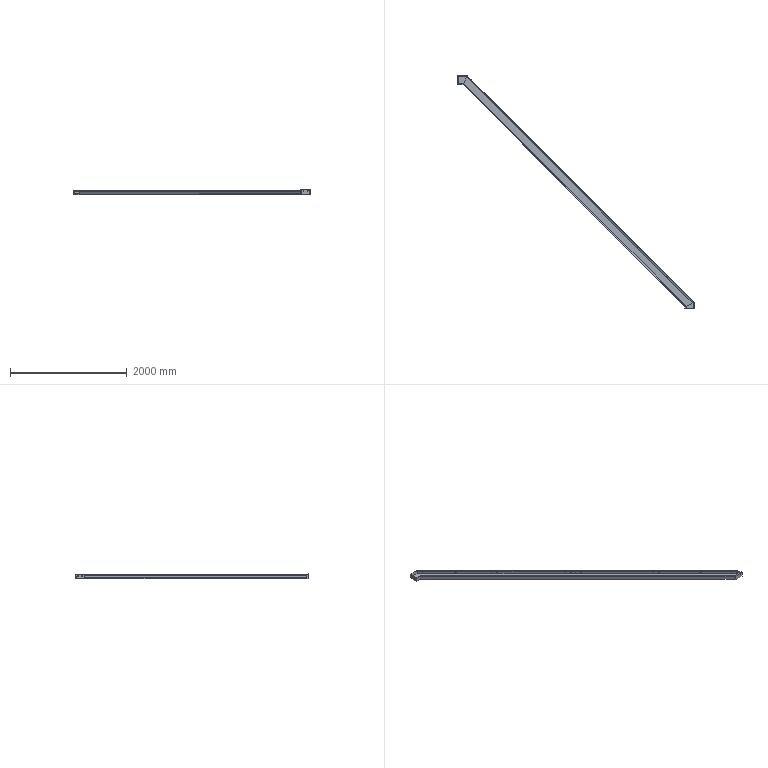Part | STEP file | PN_0051 first-floor stair beam_Default<As Machined> | 5 solids | 74 faces | box 4058 x 4000 x 90 mm | volume 12422698 mm3 | plane 42 | cylinder 32 | commonest cylinder face diameters 6.8 x12 20 x8 10 x6 16 x2 18 x2 25 x2